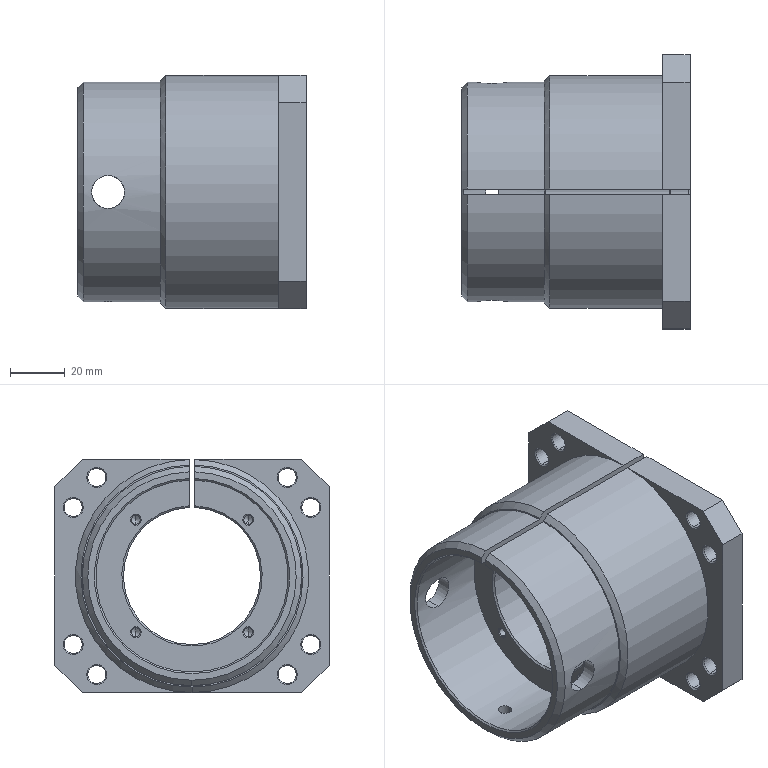Part | SolidWorks | features ICE 5, Chamfer 4, MoveFace 4, MirrorPattern 3, CirPattern 1, DelFace 1, Fillet 1, HoleWzd 1, LockFeature 1, Revolution 1 | 1 solid | 135 faces | box 83.2 x 100 x 85 mm | volume 237929 mm3 | cone 74 | cylinder 43 | plane 18 | commonest cylinder face diameters 3.3 x16 6.5 x16 12 x4 4.8 x2 70 x2 50 x1